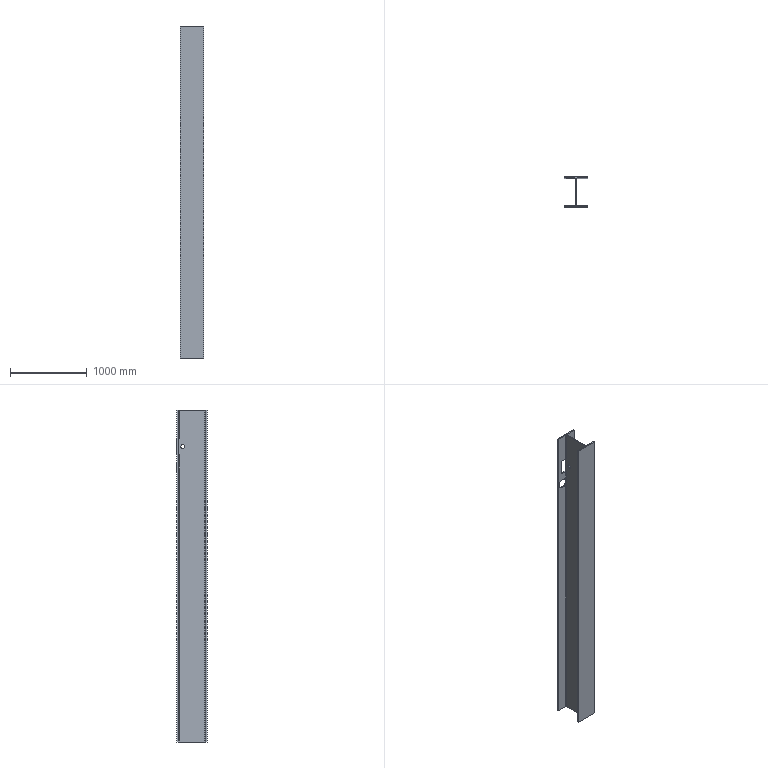Part | SolidWorks | features ICE 2, Extrusion 1 | 1 solid | 28 faces | box 300 x 390 x 4313 mm | volume 56956384 mm3 | plane 18 | cylinder 10 | commonest cylinder face diameters 26 x6 51 x2 125 x2
STEP:
#1=CARTESIAN_POINT('',(155.,289.5,3838.));
#2=VERTEX_POINT('',#1);
#3=CARTESIAN_POINT('',(155.,340.5,3838.));
#4=VERTEX_POINT('',#3);
#5=CARTESIAN_POINT('',(155.,315.,3838.));
#6=DIRECTION('',(1.,0.,0.));
#7=DIRECTION('',(0.,0.,1.));
#8=AXIS2_PLACEMENT_3D('',#5,#6,#7);
#9=CIRCLE('',#8,25.5);
#10=EDGE_CURVE('',#2,#4,#9,.T.);
#11=ORIENTED_EDGE('',*,*,#10,.T.);
#12=CARTESIAN_POINT('',(145.,340.5,3838.));
#13=VERTEX_POINT('',#12);
#14=CARTESIAN_POINT('',(300.001,340.5,3838.));
#15=DIRECTION('',(-1.,0.,0.));
#16=VECTOR('',#15,1000.);
#17=LINE('',#14,#16);
#18=EDGE_CURVE('',#4,#13,#17,.T.);
#19=ORIENTED_EDGE('',*,*,#18,.T.);
#20=CARTESIAN_POINT('',(145.,289.5,3838.));
#21=VERTEX_POINT('',#20);
#22=CARTESIAN_POINT('',(145.,315.,3838.));
#23=DIRECTION('',(-1.,0.,0.));
#24=DIRECTION('',(0.,-1.,0.));
#25=AXIS2_PLACEMENT_3D('',#22,#23,#24);
#26=CIRCLE('',#25,25.5);
#27=EDGE_CURVE('',#13,#21,#26,.T.);
#28=ORIENTED_EDGE('',*,*,#27,.T.);
#29=CARTESIAN_POINT('',(300.001,289.5,3838.));
#30=DIRECTION('',(-1.,0.,0.));
#31=VECTOR('',#30,1000.);
#32=LINE('',#29,#31);
#33=EDGE_CURVE('',#2,#21,#32,.T.);
#34=ORIENTED_EDGE('',*,*,#33,.F.);
#35=EDGE_LOOP('',(#11,#19,#28,#34));
#36=FACE_OUTER_BOUND('',#35,.T.);
#37=CARTESIAN_POINT('',(300.001,315.,3838.));
#38=DIRECTION('',(-1.,0.,0.));
#39=DIRECTION('',(0.,-1.,0.));
#40=AXIS2_PLACEMENT_3D('',#37,#38,#39);
#41=CYLINDRICAL_SURFACE('',#40,25.5);
#42=ADVANCED_FACE('',(#36),#41,.F.);
#43=CARTESIAN_POINT('',(85.,374.,3510.5));
#44=VERTEX_POINT('',#43);
#45=CARTESIAN_POINT('',(85.,374.,3635.5));
#46=VERTEX_POINT('',#45);
#47=CARTESIAN_POINT('',(85.,374.,3573.));
#48=DIRECTION('',(0.,1.,0.));
#49=DIRECTION('',(-1.,0.,0.));
#50=AXIS2_PLACEMENT_3D('',#47,#48,#49);
#51=CIRCLE('',#50,62.5);
#52=EDGE_CURVE('',#44,#46,#51,.T.);
#53=ORIENTED_EDGE('',*,*,#52,.F.);
#54=CARTESIAN_POINT('',(85.,390.,3510.5));
#55=VERTEX_POINT('',#54);
#56=CARTESIAN_POINT('',(85.,360.,3510.5));
#57=DIRECTION('',(0.,1.,0.));
#58=VECTOR('',#57,1000.);
#59=LINE('',#56,#58);
#60=EDGE_CURVE('',#44,#55,#59,.T.);
#61=ORIENTED_EDGE('',*,*,#60,.T.);
#62=CARTESIAN_POINT('',(85.,390.,3635.5));
#63=VERTEX_POINT('',#62);
#64=CARTESIAN_POINT('',(85.,390.,3573.));
#65=DIRECTION('',(0.,1.,0.));
#66=DIRECTION('',(0.,0.,1.));
#67=AXIS2_PLACEMENT_3D('',#64,#65,#66);
#68=CIRCLE('',#67,62.5);
#69=EDGE_CURVE('',#55,#63,#68,.T.);
#70=ORIENTED_EDGE('',*,*,#69,.T.);
#71=CARTESIAN_POINT('',(85.,360.,3635.5));
#72=DIRECTION('',(0.,1.,0.));
#73=VECTOR('',#72,1000.);
#74=LINE('',#71,#73);
#75=EDGE_CURVE('',#46,#63,#74,.T.);
#76=ORIENTED_EDGE('',*,*,#75,.F.);
#77=EDGE_LOOP('',(#53,#61,#70,#76));
#78=FACE_OUTER_BOUND('',#77,.T.);
#79=CARTESIAN_POINT('',(85.,360.,3573.));
#80=DIRECTION('',(0.,1.,0.));
#81=DIRECTION('',(0.,0.,1.));
#82=AXIS2_PLACEMENT_3D('',#79,#80,#81);
#83=CYLINDRICAL_SURFACE('',#82,62.5);
#84=ADVANCED_FACE('',(#78),#83,.F.);
#85=CARTESIAN_POINT('',(132.,374.,3738.));
#86=VERTEX_POINT('',#85);
#87=CARTESIAN_POINT('',(132.,374.,3614.198));
#88=VERTEX_POINT('',#87);
#89=CARTESIAN_POINT('',(132.,374.,4313.));
#90=DIRECTION('',(0.,0.,-1.));
#91=VECTOR('',#90,1000.);
#92=LINE('',#89,#91);
#93=EDGE_CURVE('',#86,#88,#92,.T.);
#94=ORIENTED_EDGE('',*,*,#93,.T.);
#95=CARTESIAN_POINT('',(145.,361.,3590.5));
#96=VERTEX_POINT('',#95);
#97=CARTESIAN_POINT('',(132.,374.,3614.198));
#98=CARTESIAN_POINT('',(132.872,374.,3613.203));
#99=CARTESIAN_POINT('',(133.708,373.913,3612.185));
#100=CARTESIAN_POINT('',(134.912,373.676,3610.623));
#101=CARTESIAN_POINT('',(135.304,373.579,3610.097));
#102=CARTESIAN_POINT('',(136.073,373.352,3609.032));
#103=CARTESIAN_POINT('',(136.447,373.222,3608.495));
#104=CARTESIAN_POINT('',(137.533,372.789,3606.885));
#105=CARTESIAN_POINT('',(138.212,372.445,3605.808));
#106=CARTESIAN_POINT('',(139.486,371.655,3603.644));
#107=CARTESIAN_POINT('',(140.082,371.21,3602.559));
#108=CARTESIAN_POINT('',(140.918,370.466,3600.925));
#109=CARTESIAN_POINT('',(141.187,370.206,3600.38));
#110=CARTESIAN_POINT('',(141.705,369.658,3599.29));
#111=CARTESIAN_POINT('',(141.955,369.369,3598.744));
#112=CARTESIAN_POINT('',(142.434,368.764,3597.657));
#113=CARTESIAN_POINT('',(142.662,368.448,3597.117));
#114=CARTESIAN_POINT('',(143.097,367.783,3596.049));
#115=CARTESIAN_POINT('',(143.305,367.433,3595.52));
#116=CARTESIAN_POINT('',(143.694,366.693,3594.483));
#117=CARTESIAN_POINT('',(143.877,366.304,3593.976));
#118=CARTESIAN_POINT('',(144.131,365.679,3593.245));
#119=CARTESIAN_POINT('',(144.212,365.463,3593.006));
#120=CARTESIAN_POINT('',(144.367,365.013,3592.54));
#121=CARTESIAN_POINT('',(144.441,364.778,3592.314));
#122=CARTESIAN_POINT('',(144.58,364.287,3591.881));
#123=CARTESIAN_POINT('',(144.645,364.032,3591.677));
#124=CARTESIAN_POINT('',(144.761,363.494,3591.299));
#125=CARTESIAN_POINT('',(144.814,363.21,3591.125));
#126=CARTESIAN_POINT('',(144.902,362.62,3590.833));
#127=CARTESIAN_POINT('',(144.938,362.313,3590.713));
#128=CARTESIAN_POINT('',(144.974,361.831,3590.588));
#129=CARTESIAN_POINT('',(144.984,361.665,3590.555));
#130=CARTESIAN_POINT('',(144.997,361.333,3590.511));
#131=CARTESIAN_POINT('',(145.,361.166,3590.5));
#132=CARTESIAN_POINT('',(145.,361.,3590.5));
#133=B_SPLINE_CURVE_WITH_KNOTS('',3,(#97,#98,#99,#100,#101,#102,#103,#104,#105,#106,#107,#108,#109,#110,#111,#112,#113,#114,#115,#116,#117,#118,#119,#120,#121,#122,#123,#124,#125,#126,#127,#128,#129,#130,#131,#132),.UNSPECIFIED.,.F.,.F.,(4,2,2,2,2,2,2,2,2,2,2,2,2,2,2,2,2,4),(0.02497,0.02896,0.03095,0.03294,0.03692,0.04091,0.0429,0.04489,0.04688,0.04888,0.05087,0.05187,0.05286,0.05386,0.05485,0.05585,0.05635,0.05685),.UNSPECIFIED.);
#134=EDGE_CURVE('',#88,#96,#133,.T.);
#135=ORIENTED_EDGE('',*,*,#134,.T.);
#136=CARTESIAN_POINT('',(145.,361.,3738.));
#137=VERTEX_POINT('',#136);
#138=CARTESIAN_POINT('',(145.,361.,4313.));
#139=DIRECTION('',(0.,0.,-1.));
#140=VECTOR('',#139,1000.);
#141=LINE('',#138,#140);
#142=EDGE_CURVE('',#137,#96,#141,.T.);
#143=ORIENTED_EDGE('',*,*,#142,.F.);
#144=CARTESIAN_POINT('',(132.,361.,3738.));
#145=DIRECTION('',(0.,0.,1.));
#146=DIRECTION('',(-1.,0.,0.));
#147=AXIS2_PLACEMENT_3D('',#144,#145,#146);
#148=CIRCLE('',#147,13.);
#149=EDGE_CURVE('',#137,#86,#148,.T.);
#150=ORIENTED_EDGE('',*,*,#149,.T.);
#151=EDGE_LOOP('',(#94,#135,#143,#150));
#152=FACE_OUTER_BOUND('',#151,.T.);
#153=CARTESIAN_POINT('',(132.,361.,4313.));
#154=DIRECTION('',(0.,0.,-1.));
#155=DIRECTION('',(-1.,0.,0.));
#156=AXIS2_PLACEMENT_3D('',#153,#154,#155);
#157=CYLINDRICAL_SURFACE('',#156,13.);
#158=ADVANCED_FACE('',(#152),#157,.F.);
#159=CARTESIAN_POINT('',(132.,374.,4313.));
#160=VERTEX_POINT('',#159);
#161=CARTESIAN_POINT('',(132.,374.,3938.));
#162=VERTEX_POINT('',#161);
#163=CARTESIAN_POINT('',(132.,374.,4313.));
#164=DIRECTION('',(0.,0.,-1.));
#165=VECTOR('',#164,1000.);
#166=LINE('',#163,#165);
#167=EDGE_CURVE('',#160,#162,#166,.T.);
#168=ORIENTED_EDGE('',*,*,#167,.T.);
#169=CARTESIAN_POINT('',(145.,361.,3938.));
#170=VERTEX_POINT('',#169);
#171=CARTESIAN_POINT('',(132.,361.,3938.));
#172=DIRECTION('',(0.,0.,-1.));
#173=DIRECTION('',(1.,0.,0.));
#174=AXIS2_PLACEMENT_3D('',#171,#172,#173);
#175=CIRCLE('',#174,13.);
#176=EDGE_CURVE('',#162,#170,#175,.T.);
#177=ORIENTED_EDGE('',*,*,#176,.T.);
#178=CARTESIAN_POINT('',(145.,361.,4313.));
#179=VERTEX_POINT('',#178);
#180=CARTESIAN_POINT('',(145.,361.,4313.));
#181=DIRECTION('',(0.,0.,-1.));
#182=VECTOR('',#181,1000.);
#183=LINE('',#180,#182);
#184=EDGE_CURVE('',#179,#170,#183,.T.);
#185=ORIENTED_EDGE('',*,*,#184,.F.);
#186=CARTESIAN_POINT('',(132.,361.,4313.));
#187=DIRECTION('',(0.,0.,-1.));
#188=DIRECTION('',(-1.,0.,0.));
#189=AXIS2_PLACEMENT_3D('',#186,#187,#188);
#190=CIRCLE('',#189,13.);
#191=EDGE_CURVE('',#160,#179,#190,.T.);
#192=ORIENTED_EDGE('',*,*,#191,.F.);
#193=EDGE_LOOP('',(#168,#177,#185,#192));
#194=FACE_OUTER_BOUND('',#193,.T.);
#195=CARTESIAN_POINT('',(132.,361.,4313.));
#196=DIRECTION('',(0.,0.,-1.));
#197=DIRECTION('',(-1.,0.,0.));
#198=AXIS2_PLACEMENT_3D('',#195,#196,#197);
#199=CYLINDRICAL_SURFACE('',#198,13.);
#200=ADVANCED_FACE('',(#194),#199,.F.);
#201=CARTESIAN_POINT('',(0.,16.,0.));
#202=VERTEX_POINT('',#201);
#203=CARTESIAN_POINT('',(0.,0.,0.));
#204=VERTEX_POINT('',#203);
#205=CARTESIAN_POINT('',(0.,16.,0.));
#206=DIRECTION('',(0.,-1.,0.));
#207=VECTOR('',#206,1000.);
#208=LINE('',#205,#207);
#209=EDGE_CURVE('',#202,#204,#208,.T.);
#210=ORIENTED_EDGE('',*,*,#209,.T.);
#211=CARTESIAN_POINT('',(0.,0.,4313.));
#212=VERTEX_POINT('',#211);
#213=CARTESIAN_POINT('',(0.,0.,4313.));
#214=DIRECTION('',(0.,0.,-1.));
#215=VECTOR('',#214,1000.);
#216=LINE('',#213,#215);
#217=EDGE_CURVE('',#212,#204,#216,.T.);
#218=ORIENTED_EDGE('',*,*,#217,.F.);
#219=CARTESIAN_POINT('',(0.,16.,4313.));
#220=VERTEX_POINT('',#219);
#221=CARTESIAN_POINT('',(0.,16.,4313.));
#222=DIRECTION('',(0.,-1.,0.));
#223=VECTOR('',#222,1000.);
#224=LINE('',#221,#223);
#225=EDGE_CURVE('',#220,#212,#224,.T.);
#226=ORIENTED_EDGE('',*,*,#225,.F.);
#227=CARTESIAN_POINT('',(0.,16.,4313.));
#228=DIRECTION('',(0.,0.,-1.));
#229=VECTOR('',#228,1000.);
#230=LINE('',#227,#229);
#231=EDGE_CURVE('',#220,#202,#230,.T.);
#232=ORIENTED_EDGE('',*,*,#231,.T.);
#233=EDGE_LOOP('',(#210,#218,#226,#232));
#234=FACE_OUTER_BOUND('',#233,.T.);
#235=CARTESIAN_POINT('',(0.,16.,4313.));
#236=DIRECTION('',(1.,0.,0.));
#237=DIRECTION('',(0.,1.,0.));
#238=AXIS2_PLACEMENT_3D('',#235,#236,#237);
#239=PLANE('',#238);
#240=ADVANCED_FACE('',(#234),#239,.F.);
#241=CARTESIAN_POINT('',(300.,0.,0.));
#242=VERTEX_POINT('',#241);
#243=CARTESIAN_POINT('',(0.,0.,0.));
#244=DIRECTION('',(1.,0.,0.));
#245=VECTOR('',#244,1000.);
#246=LINE('',#243,#245);
#247=EDGE_CURVE('',#204,#242,#246,.T.);
#248=ORIENTED_EDGE('',*,*,#247,.T.);
#249=CARTESIAN_POINT('',(300.,0.,4313.));
#250=VERTEX_POINT('',#249);
#251=CARTESIAN_POINT('',(300.,0.,4313.));
#252=DIRECTION('',(0.,0.,-1.));
#253=VECTOR('',#252,1000.);
#254=LINE('',#251,#253);
#255=EDGE_CURVE('',#250,#242,#254,.T.);
#256=ORIENTED_EDGE('',*,*,#255,.F.);
#257=CARTESIAN_POINT('',(0.,0.,4313.));
#258=DIRECTION('',(1.,0.,0.));
#259=VECTOR('',#258,1000.);
#260=LINE('',#257,#259);
#261=EDGE_CURVE('',#212,#250,#260,.T.);
#262=ORIENTED_EDGE('',*,*,#261,.F.);
#263=ORIENTED_EDGE('',*,*,#217,.T.);
#264=EDGE_LOOP('',(#248,#256,#262,#263));
#265=FACE_OUTER_BOUND('',#264,.T.);
#266=CARTESIAN_POINT('',(0.,0.,4313.));
#267=DIRECTION('',(0.,1.,0.));
#268=DIRECTION('',(0.,0.,1.));
#269=AXIS2_PLACEMENT_3D('',#266,#267,#268);
#270=PLANE('',#269);
#271=ADVANCED_FACE('',(#265),#270,.F.);
#272=CARTESIAN_POINT('',(300.,16.,0.));
#273=VERTEX_POINT('',#272);
#274=CARTESIAN_POINT('',(300.,0.,0.));
#275=DIRECTION('',(0.,1.,0.));
#276=VECTOR('',#275,1000.);
#277=LINE('',#274,#276);
#278=EDGE_CURVE('',#242,#273,#277,.T.);
#279=ORIENTED_EDGE('',*,*,#278,.T.);
#280=CARTESIAN_POINT('',(300.,16.,4313.));
#281=VERTEX_POINT('',#280);
#282=CARTESIAN_POINT('',(300.,16.,4313.));
#283=DIRECTION('',(0.,0.,-1.));
#284=VECTOR('',#283,1000.);
#285=LINE('',#282,#284);
#286=EDGE_CURVE('',#281,#273,#285,.T.);
#287=ORIENTED_EDGE('',*,*,#286,.F.);
#288=CARTESIAN_POINT('',(300.,0.,4313.));
#289=DIRECTION('',(0.,1.,0.));
#290=VECTOR('',#289,1000.);
#291=LINE('',#288,#290);
#292=EDGE_CURVE('',#250,#281,#291,.T.);
#293=ORIENTED_EDGE('',*,*,#292,.F.);
#294=ORIENTED_EDGE('',*,*,#255,.T.);
#295=EDGE_LOOP('',(#279,#287,#293,#294));
#296=FACE_OUTER_BOUND('',#295,.T.);
#297=CARTESIAN_POINT('',(300.,0.,4313.));
#298=DIRECTION('',(-1.,0.,0.));
#299=DIRECTION('',(0.,0.,1.));
#300=AXIS2_PLACEMENT_3D('',#297,#298,#299);
#301=PLANE('',#300);
#302=ADVANCED_FACE('',(#296),#301,.F.);
#303=CARTESIAN_POINT('',(168.,16.,0.));
#304=VERTEX_POINT('',#303);
#305=CARTESIAN_POINT('',(300.,16.,0.));
#306=DIRECTION('',(-1.,0.,0.));
#307=VECTOR('',#306,1000.);
#308=LINE('',#305,#307);
#309=EDGE_CURVE('',#273,#304,#308,.T.);
#310=ORIENTED_EDGE('',*,*,#309,.T.);
#311=CARTESIAN_POINT('',(168.,16.,4313.));
#312=VERTEX_POINT('',#311);
#313=CARTESIAN_POINT('',(168.,16.,4313.));
#314=DIRECTION('',(0.,0.,-1.));
#315=VECTOR('',#314,1000.);
#316=LINE('',#313,#315);
#317=EDGE_CURVE('',#312,#304,#316,.T.);
#318=ORIENTED_EDGE('',*,*,#317,.F.);
#319=CARTESIAN_POINT('',(300.,16.,4313.));
#320=DIRECTION('',(-1.,0.,0.));
#321=VECTOR('',#320,1000.);
#322=LINE('',#319,#321);
#323=EDGE_CURVE('',#281,#312,#322,.T.);
#324=ORIENTED_EDGE('',*,*,#323,.F.);
#325=ORIENTED_EDGE('',*,*,#286,.T.);
#326=EDGE_LOOP('',(#310,#318,#324,#325));
#327=FACE_OUTER_BOUND('',#326,.T.);
#328=CARTESIAN_POINT('',(300.,16.,4313.));
#329=DIRECTION('',(0.,-1.,0.));
#330=DIRECTION('',(1.,0.,0.));
#331=AXIS2_PLACEMENT_3D('',#328,#329,#330);
#332=PLANE('',#331);
#333=ADVANCED_FACE('',(#327),#332,.F.);
#334=CARTESIAN_POINT('',(155.,29.,0.));
#335=VERTEX_POINT('',#334);
#336=CARTESIAN_POINT('',(168.,29.,0.));
#337=DIRECTION('',(0.,0.,-1.));
#338=DIRECTION('',(-1.,0.,0.));
#339=AXIS2_PLACEMENT_3D('',#336,#337,#338);
#340=CIRCLE('',#339,13.);
#341=EDGE_CURVE('',#304,#335,#340,.T.);
#342=ORIENTED_EDGE('',*,*,#341,.T.);
#343=CARTESIAN_POINT('',(155.,29.,4313.));
#344=VERTEX_POINT('',#343);
#345=CARTESIAN_POINT('',(155.,29.,4313.));
#346=DIRECTION('',(0.,0.,-1.));
#347=VECTOR('',#346,1000.);
#348=LINE('',#345,#347);
#349=EDGE_CURVE('',#344,#335,#348,.T.);
#350=ORIENTED_EDGE('',*,*,#349,.F.);
#351=CARTESIAN_POINT('',(168.,29.,4313.));
#352=DIRECTION('',(0.,0.,-1.));
#353=DIRECTION('',(-1.,0.,0.));
#354=AXIS2_PLACEMENT_3D('',#351,#352,#353);
#355=CIRCLE('',#354,13.);
#356=EDGE_CURVE('',#312,#344,#355,.T.);
#357=ORIENTED_EDGE('',*,*,#356,.F.);
#358=ORIENTED_EDGE('',*,*,#317,.T.);
#359=EDGE_LOOP('',(#342,#350,#357,#358));
#360=FACE_OUTER_BOUND('',#359,.T.);
#361=CARTESIAN_POINT('',(168.,29.,4313.));
#362=DIRECTION('',(0.,0.,-1.));
#363=DIRECTION('',(-1.,0.,0.));
#364=AXIS2_PLACEMENT_3D('',#361,#362,#363);
#365=CYLINDRICAL_SURFACE('',#364,13.);
#366=ADVANCED_FACE('',(#360),#365,.F.);
#367=ORIENTED_EDGE('',*,*,#10,.F.);
#368=CARTESIAN_POINT('',(155.,315.,3838.));
#369=DIRECTION('',(1.,0.,0.));
#370=DIRECTION('',(0.,0.,1.));
#371=AXIS2_PLACEMENT_3D('',#368,#369,#370);
#372=CIRCLE('',#371,25.5);
#373=EDGE_CURVE('',#4,#2,#372,.T.);
#374=ORIENTED_EDGE('',*,*,#373,.F.);
#375=EDGE_LOOP('',(#367,#374));
#376=FACE_BOUND('',#375,.T.);
#377=CARTESIAN_POINT('',(155.,361.,0.));
#378=VERTEX_POINT('',#377);
#379=CARTESIAN_POINT('',(155.,29.,0.));
#380=DIRECTION('',(0.,1.,0.));
#381=VECTOR('',#380,1000.);
#382=LINE('',#379,#381);
#383=EDGE_CURVE('',#335,#378,#382,.T.);
#384=ORIENTED_EDGE('',*,*,#383,.T.);
#385=CARTESIAN_POINT('',(155.,361.,4313.));
#386=VERTEX_POINT('',#385);
#387=CARTESIAN_POINT('',(155.,361.,4313.));
#388=DIRECTION('',(0.,0.,-1.));
#389=VECTOR('',#388,1000.);
#390=LINE('',#387,#389);
#391=EDGE_CURVE('',#386,#378,#390,.T.);
#392=ORIENTED_EDGE('',*,*,#391,.F.);
#393=CARTESIAN_POINT('',(155.,29.,4313.));
#394=DIRECTION('',(0.,1.,0.));
#395=VECTOR('',#394,1000.);
#396=LINE('',#393,#395);
#397=EDGE_CURVE('',#344,#386,#396,.T.);
#398=ORIENTED_EDGE('',*,*,#397,.F.);
#399=ORIENTED_EDGE('',*,*,#349,.T.);
#400=EDGE_LOOP('',(#384,#392,#398,#399));
#401=FACE_OUTER_BOUND('',#400,.T.);
#402=CARTESIAN_POINT('',(155.,29.,4313.));
#403=DIRECTION('',(-1.,0.,0.));
#404=DIRECTION('',(0.,0.,1.));
#405=AXIS2_PLACEMENT_3D('',#402,#403,#404);
#406=PLANE('',#405);
#407=ADVANCED_FACE('',(#376,#401),#406,.F.);
#408=CARTESIAN_POINT('',(168.,374.,0.));
#409=VERTEX_POINT('',#408);
#410=CARTESIAN_POINT('',(168.,361.,0.));
#411=DIRECTION('',(0.,0.,-1.));
#412=DIRECTION('',(-1.,0.,0.));
#413=AXIS2_PLACEMENT_3D('',#410,#411,#412);
#414=CIRCLE('',#413,13.);
#415=EDGE_CURVE('',#378,#409,#414,.T.);
#416=ORIENTED_EDGE('',*,*,#415,.T.);
#417=CARTESIAN_POINT('',(168.,374.,4313.));
#418=VERTEX_POINT('',#417);
#419=CARTESIAN_POINT('',(168.,374.,4313.));
#420=DIRECTION('',(0.,0.,-1.));
#421=VECTOR('',#420,1000.);
#422=LINE('',#419,#421);
#423=EDGE_CURVE('',#418,#409,#422,.T.);
#424=ORIENTED_EDGE('',*,*,#423,.F.);
#425=CARTESIAN_POINT('',(168.,361.,4313.));
#426=DIRECTION('',(0.,0.,-1.));
#427=DIRECTION('',(-1.,0.,0.));
#428=AXIS2_PLACEMENT_3D('',#425,#426,#427);
#429=CIRCLE('',#428,13.);
#430=EDGE_CURVE('',#386,#418,#429,.T.);
#431=ORIENTED_EDGE('',*,*,#430,.F.);
#432=ORIENTED_EDGE('',*,*,#391,.T.);
#433=EDGE_LOOP('',(#416,#424,#431,#432));
#434=FACE_OUTER_BOUND('',#433,.T.);
#435=CARTESIAN_POINT('',(168.,361.,4313.));
#436=DIRECTION('',(0.,0.,-1.));
#437=DIRECTION('',(-1.,0.,0.));
#438=AXIS2_PLACEMENT_3D('',#435,#436,#437);
#439=CYLINDRICAL_SURFACE('',#438,13.);
#440=ADVANCED_FACE('',(#434),#439,.F.);
#441=CARTESIAN_POINT('',(300.,374.,0.));
#442=VERTEX_POINT('',#441);
#443=CARTESIAN_POINT('',(168.,374.,0.));
#444=DIRECTION('',(1.,0.,0.));
#445=VECTOR('',#444,1000.);
#446=LINE('',#443,#445);
#447=EDGE_CURVE('',#409,#442,#446,.T.);
#448=ORIENTED_EDGE('',*,*,#447,.T.);
#449=CARTESIAN_POINT('',(300.,374.,4313.));
#450=VERTEX_POINT('',#449);
#451=CARTESIAN_POINT('',(300.,374.,4313.));
#452=DIRECTION('',(0.,0.,-1.));
#453=VECTOR('',#452,1000.);
#454=LINE('',#451,#453);
#455=EDGE_CURVE('',#450,#442,#454,.T.);
#456=ORIENTED_EDGE('',*,*,#455,.F.);
#457=CARTESIAN_POINT('',(168.,374.,4313.));
#458=DIRECTION('',(1.,0.,0.));
#459=VECTOR('',#458,1000.);
#460=LINE('',#457,#459);
#461=EDGE_CURVE('',#418,#450,#460,.T.);
#462=ORIENTED_EDGE('',*,*,#461,.F.);
#463=ORIENTED_EDGE('',*,*,#423,.T.);
#464=EDGE_LOOP('',(#448,#456,#462,#463));
#465=FACE_OUTER_BOUND('',#464,.T.);
#466=CARTESIAN_POINT('',(168.,374.,4313.));
#467=DIRECTION('',(0.,1.,0.));
#468=DIRECTION('',(0.,0.,1.));
#469=AXIS2_PLACEMENT_3D('',#466,#467,#468);
#470=PLANE('',#469);
#471=ADVANCED_FACE('',(#465),#470,.F.);
#472=CARTESIAN_POINT('',(300.,390.,0.));
#473=VERTEX_POINT('',#472);
#474=CARTESIAN_POINT('',(300.,374.,0.));
#475=DIRECTION('',(0.,1.,0.));
#476=VECTOR('',#475,1000.);
#477=LINE('',#474,#476);
#478=EDGE_CURVE('',#442,#473,#477,.T.);
#479=ORIENTED_EDGE('',*,*,#478,.T.);
#480=CARTESIAN_POINT('',(300.,390.,4313.));
#481=VERTEX_POINT('',#480);
#482=CARTESIAN_POINT('',(300.,390.,4313.));
#483=DIRECTION('',(0.,0.,-1.));
#484=VECTOR('',#483,1000.);
#485=LINE('',#482,#484);
#486=EDGE_CURVE('',#481,#473,#485,.T.);
#487=ORIENTED_EDGE('',*,*,#486,.F.);
#488=CARTESIAN_POINT('',(300.,374.,4313.));
#489=DIRECTION('',(0.,1.,0.));
#490=VECTOR('',#489,1000.);
#491=LINE('',#488,#490);
#492=EDGE_CURVE('',#450,#481,#491,.T.);
#493=ORIENTED_EDGE('',*,*,#492,.F.);
#494=ORIENTED_EDGE('',*,*,#455,.T.);
#495=EDGE_LOOP('',(#479,#487,#493,#494));
#496=FACE_OUTER_BOUND('',#495,.T.);
#497=CARTESIAN_POINT('',(300.,374.,4313.));
#498=DIRECTION('',(-1.,0.,0.));
#499=DIRECTION('',(0.,-1.,0.));
#500=AXIS2_PLACEMENT_3D('',#497,#498,#499);
#501=PLANE('',#500);
#502=ADVANCED_FACE('',(#496),#501,.F.);
#503=CARTESIAN_POINT('',(85.,390.,3573.));
#504=DIRECTION('',(0.,1.,0.));
#505=DIRECTION('',(0.,0.,1.));
#506=AXIS2_PLACEMENT_3D('',#503,#504,#505);
#507=CIRCLE('',#506,62.5);
#508=EDGE_CURVE('',#63,#55,#507,.T.);
#509=ORIENTED_EDGE('',*,*,#508,.F.);
#510=ORIENTED_EDGE('',*,*,#69,.F.);
#511=EDGE_LOOP('',(#509,#510));
#512=FACE_BOUND('',#511,.T.);
#513=CARTESIAN_POINT('',(145.,390.,3738.));
#514=VERTEX_POINT('',#513);
#515=CARTESIAN_POINT('',(55.,390.,3738.));
#516=VERTEX_POINT('',#515);
#517=CARTESIAN_POINT('',(145.,390.,3738.));
#518=DIRECTION('',(-1.,0.,0.));
#519=VECTOR('',#518,1000.);
#520=LINE('',#517,#519);
#521=EDGE_CURVE('',#514,#516,#520,.T.);
#522=ORIENTED_EDGE('',*,*,#521,.F.);
#523=CARTESIAN_POINT('',(145.,390.,3938.));
#524=VERTEX_POINT('',#523);
#525=CARTESIAN_POINT('',(145.,390.,3738.));
#526=DIRECTION('',(0.,0.,-1.));
#527=VECTOR('',#526,1000.);
#528=LINE('',#525,#527);
#529=EDGE_CURVE('',#524,#514,#528,.T.);
#530=ORIENTED_EDGE('',*,*,#529,.F.);
#531=CARTESIAN_POINT('',(55.,390.,3938.));
#532=VERTEX_POINT('',#531);
#533=CARTESIAN_POINT('',(145.,390.,3938.));
#534=DIRECTION('',(1.,0.,0.));
#535=VECTOR('',#534,1000.);
#536=LINE('',#533,#535);
#537=EDGE_CURVE('',#532,#524,#536,.T.);
#538=ORIENTED_EDGE('',*,*,#537,.F.);
#539=CARTESIAN_POINT('',(55.,390.,3738.));
#540=DIRECTION('',(0.,0.,1.));
#541=VECTOR('',#540,1000.);
#542=LINE('',#539,#541);
#543=EDGE_CURVE('',#516,#532,#542,.T.);
#544=ORIENTED_EDGE('',*,*,#543,.F.);
#545=EDGE_LOOP('',(#522,#530,#538,#544));
#546=FACE_BOUND('',#545,.T.);
#547=CARTESIAN_POINT('',(0.,390.,0.));
#548=VERTEX_POINT('',#547);
#549=CARTESIAN_POINT('',(300.,390.,0.));
#550=DIRECTION('',(-1.,0.,0.));
#551=VECTOR('',#550,1000.);
#552=LINE('',#549,#551);
#553=EDGE_CURVE('',#473,#548,#552,.T.);
#554=ORIENTED_EDGE('',*,*,#553,.T.);
#555=CARTESIAN_POINT('',(0.,390.,4313.));
#556=VERTEX_POINT('',#555);
#557=CARTESIAN_POINT('',(0.,390.,4313.));
#558=DIRECTION('',(0.,0.,-1.));
#559=VECTOR('',#558,1000.);
#560=LINE('',#557,#559);
#561=EDGE_CURVE('',#556,#548,#560,.T.);
#562=ORIENTED_EDGE('',*,*,#561,.F.);
#563=CARTESIAN_POINT('',(300.,390.,4313.));
#564=DIRECTION('',(-1.,0.,0.));
#565=VECTOR('',#564,1000.);
#566=LINE('',#563,#565);
#567=EDGE_CURVE('',#481,#556,#566,.T.);
#568=ORIENTED_EDGE('',*,*,#567,.F.);
#569=ORIENTED_EDGE('',*,*,#486,.T.);
#570=EDGE_LOOP('',(#554,#562,#568,#569));
#571=FACE_OUTER_BOUND('',#570,.T.);
#572=CARTESIAN_POINT('',(300.,390.,4313.));
#573=DIRECTION('',(0.,-1.,0.));
#574=DIRECTION('',(0.,0.,-1.));
#575=AXIS2_PLACEMENT_3D('',#572,#573,#574);
#576=PLANE('',#575);
#577=ADVANCED_FACE('',(#512,#546,#571),#576,.F.);
#578=CARTESIAN_POINT('',(0.,374.,0.));
#579=VERTEX_POINT('',#578);
#580=CARTESIAN_POINT('',(0.,390.,0.));
#581=DIRECTION('',(0.,-1.,0.));
#582=VECTOR('',#581,1000.);
#583=LINE('',#580,#582);
#584=EDGE_CURVE('',#548,#579,#583,.T.);
#585=ORIENTED_EDGE('',*,*,#584,.T.);
#586=CARTESIAN_POINT('',(0.,374.,4313.));
#587=VERTEX_POINT('',#586);
#588=CARTESIAN_POINT('',(0.,374.,4313.));
#589=DIRECTION('',(0.,0.,-1.));
#590=VECTOR('',#589,1000.);
#591=LINE('',#588,#590);
#592=EDGE_CURVE('',#587,#579,#591,.T.);
#593=ORIENTED_EDGE('',*,*,#592,.F.);
#594=CARTESIAN_POINT('',(0.,390.,4313.));
#595=DIRECTION('',(0.,-1.,0.));
#596=VECTOR('',#595,1000.);
#597=LINE('',#594,#596);
#598=EDGE_CURVE('',#556,#587,#597,.T.);
#599=ORIENTED_EDGE('',*,*,#598,.F.);
#600=ORIENTED_EDGE('',*,*,#561,.T.);
#601=EDGE_LOOP('',(#585,#593,#599,#600));
#602=FACE_OUTER_BOUND('',#601,.T.);
#603=CARTESIAN_POINT('',(0.,390.,4313.));
#604=DIRECTION('',(1.,0.,0.));
#605=DIRECTION('',(0.,0.,-1.));
#606=AXIS2_PLACEMENT_3D('',#603,#604,#605);
#607=PLANE('',#606);
#608=ADVANCED_FACE('',(#602),#607,.F.);
#609=CARTESIAN_POINT('',(132.,374.,3531.802));
#610=VERTEX_POINT('',#609);
#611=CARTESIAN_POINT('',(132.,374.,0.));
#612=VERTEX_POINT('',#611);
#613=CARTESIAN_POINT('',(132.,374.,4313.));
#614=DIRECTION('',(0.,0.,-1.));
#615=VECTOR('',#614,1000.);
#616=LINE('',#613,#615);
#617=EDGE_CURVE('',#610,#612,#616,.T.);
#618=ORIENTED_EDGE('',*,*,#617,.F.);
#619=CARTESIAN_POINT('',(85.,374.,3573.));
#620=DIRECTION('',(0.,1.,0.));
#621=DIRECTION('',(-1.,0.,0.));
#622=AXIS2_PLACEMENT_3D('',#619,#620,#621);
#623=CIRCLE('',#622,62.5);
#624=EDGE_CURVE('',#610,#44,#623,.T.);
#625=ORIENTED_EDGE('',*,*,#624,.T.);
#626=ORIENTED_EDGE('',*,*,#52,.T.);
#627=CARTESIAN_POINT('',(85.,374.,3573.));
#628=DIRECTION('',(0.,1.,0.));
#629=DIRECTION('',(-1.,0.,0.));
#630=AXIS2_PLACEMENT_3D('',#627,#628,#629);
#631=CIRCLE('',#630,62.5);
#632=EDGE_CURVE('',#46,#88,#631,.T.);
#633=ORIENTED_EDGE('',*,*,#632,.T.);
#634=ORIENTED_EDGE('',*,*,#93,.F.);
#635=CARTESIAN_POINT('',(55.,374.,3738.));
#636=VERTEX_POINT('',#635);
#637=CARTESIAN_POINT('',(0.,374.,3738.));
#638=DIRECTION('',(-1.,0.,0.));
#639=VECTOR('',#638,1000.);
#640=LINE('',#637,#639);
#641=EDGE_CURVE('',#86,#636,#640,.T.);
#642=ORIENTED_EDGE('',*,*,#641,.T.);
#643=CARTESIAN_POINT('',(55.,374.,3938.));
#644=VERTEX_POINT('',#643);
#645=CARTESIAN_POINT('',(55.,374.,4313.));
#646=DIRECTION('',(0.,0.,1.));
#647=VECTOR('',#646,1000.);
#648=LINE('',#645,#647);
#649=EDGE_CURVE('',#636,#644,#648,.T.);
#650=ORIENTED_EDGE('',*,*,#649,.T.);
#651=CARTESIAN_POINT('',(0.,374.,3938.));
#652=DIRECTION('',(1.,0.,0.));
#653=VECTOR('',#652,1000.);
#654=LINE('',#651,#653);
#655=EDGE_CURVE('',#644,#162,#654,.T.);
#656=ORIENTED_EDGE('',*,*,#655,.T.);
#657=ORIENTED_EDGE('',*,*,#167,.F.);
#658=CARTESIAN_POINT('',(0.,374.,4313.));
#659=DIRECTION('',(1.,0.,0.));
#660=VECTOR('',#659,1000.);
#661=LINE('',#658,#660);
#662=EDGE_CURVE('',#587,#160,#661,.T.);
#663=ORIENTED_EDGE('',*,*,#662,.F.);
#664=ORIENTED_EDGE('',*,*,#592,.T.);
#665=CARTESIAN_POINT('',(0.,374.,0.));
#666=DIRECTION('',(1.,0.,0.));
#667=VECTOR('',#666,1000.);
#668=LINE('',#665,#667);
#669=EDGE_CURVE('',#579,#612,#668,.T.);
#670=ORIENTED_EDGE('',*,*,#669,.T.);
#671=EDGE_LOOP('',(#618,#625,#626,#633,#634,#642,#650,#656,#657,#663,#664,#670));
#672=FACE_OUTER_BOUND('',#671,.T.);
#673=CARTESIAN_POINT('',(0.,374.,4313.));
#674=DIRECTION('',(0.,1.,0.));
#675=DIRECTION('',(-1.,0.,0.));
#676=AXIS2_PLACEMENT_3D('',#673,#674,#675);
#677=PLANE('',#676);
#678=ADVANCED_FACE('',(#672),#677,.F.);
#679=CARTESIAN_POINT('',(145.,361.,3555.5));
#680=VERTEX_POINT('',#679);
#681=CARTESIAN_POINT('',(145.,361.,0.));
#682=VERTEX_POINT('',#681);
#683=CARTESIAN_POINT('',(145.,361.,4313.));
#684=DIRECTION('',(0.,0.,-1.));
#685=VECTOR('',#684,1000.);
#686=LINE('',#683,#685);
#687=EDGE_CURVE('',#680,#682,#686,.T.);
#688=ORIENTED_EDGE('',*,*,#687,.F.);
#689=CARTESIAN_POINT('',(145.,361.,3555.5));
#690=CARTESIAN_POINT('',(145.,361.168,3555.5));
#691=CARTESIAN_POINT('',(144.997,361.338,3555.489));
#692=CARTESIAN_POINT('',(144.984,361.672,3555.444));
#693=CARTESIAN_POINT('',(144.974,361.837,3555.411));
#694=CARTESIAN_POINT('',(144.937,362.322,3555.284));
#695=CARTESIAN_POINT('',(144.9,362.638,3555.16));
#696=CARTESIAN_POINT('',(144.81,363.232,3554.862));
#697=CARTESIAN_POINT('',(144.758,363.513,3554.689));
#698=CARTESIAN_POINT('',(144.64,364.051,3554.308));
#699=CARTESIAN_POINT('',(144.574,364.31,3554.1));
#700=CARTESIAN_POINT('',(144.365,365.046,3553.449));
#701=CARTESIAN_POINT('',(144.209,365.488,3552.979));
#702=CARTESIAN_POINT('',(143.87,366.321,3552.003));
#703=CARTESIAN_POINT('',(143.687,366.709,3551.496));
#704=CARTESIAN_POINT('',(143.296,367.448,3550.458));
#705=CARTESIAN_POINT('',(143.088,367.798,3549.927));
#706=CARTESIAN_POINT('',(142.653,368.462,3548.86));
#707=CARTESIAN_POINT('',(142.425,368.776,3548.323));
#708=CARTESIAN_POINT('',(141.712,369.676,3546.705));
#709=CARTESIAN_POINT('',(141.196,370.22,3545.617));
#710=CARTESIAN_POINT('',(140.079,371.212,3543.435));
#711=CARTESIAN_POINT('',(139.478,371.661,3542.34));
#712=CARTESIAN_POINT('',(138.185,372.46,3540.149));
#713=CARTESIAN_POINT('',(137.503,372.803,3539.069));
#714=CARTESIAN_POINT('',(136.064,373.373,3536.94));
#715=CARTESIAN_POINT('',(135.308,373.598,3535.891));
#716=CARTESIAN_POINT('',(133.715,373.912,3533.824));
#717=CARTESIAN_POINT('',(132.879,374.,3532.806));
#718=CARTESIAN_POINT('',(132.,374.,3531.802));
#719=B_SPLINE_CURVE_WITH_KNOTS('',3,(#689,#690,#691,#692,#693,#694,#695,#696,#697,#698,#699,#700,#701,#702,#703,#704,#705,#706,#707,#708,#709,#710,#711,#712,#713,#714,#715,#716,#717,#718),.UNSPECIFIED.,.F.,.F.,(4,2,2,2,2,2,2,2,2,2,2,2,2,2,4),(0.001009,0.00151,0.002012,0.003016,0.00402,0.005023,0.007031,0.009038,0.01105,0.01305,0.01707,0.02108,0.0251,0.02911,0.03313),.UNSPECIFIED.);
#720=EDGE_CURVE('',#680,#610,#719,.T.);
#721=ORIENTED_EDGE('',*,*,#720,.T.);
#722=ORIENTED_EDGE('',*,*,#617,.T.);
#723=CARTESIAN_POINT('',(132.,361.,0.));
#724=DIRECTION('',(0.,0.,-1.));
#725=DIRECTION('',(-1.,0.,0.));
#726=AXIS2_PLACEMENT_3D('',#723,#724,#725);
#727=CIRCLE('',#726,13.);
#728=EDGE_CURVE('',#612,#682,#727,.T.);
#729=ORIENTED_EDGE('',*,*,#728,.T.);
#730=EDGE_LOOP('',(#688,#721,#722,#729));
#731=FACE_OUTER_BOUND('',#730,.T.);
#732=CARTESIAN_POINT('',(132.,361.,4313.));
#733=DIRECTION('',(0.,0.,-1.));
#734=DIRECTION('',(-1.,0.,0.));
#735=AXIS2_PLACEMENT_3D('',#732,#733,#734);
#736=CYLINDRICAL_SURFACE('',#735,13.);
#737=ADVANCED_FACE('',(#731),#736,.F.);
#738=CARTESIAN_POINT('',(145.,315.,3838.));
#739=DIRECTION('',(-1.,0.,0.));
#740=DIRECTION('',(0.,-1.,0.));
#741=AXIS2_PLACEMENT_3D('',#738,#739,#740);
#742=CIRCLE('',#741,25.5);
#743=EDGE_CURVE('',#21,#13,#742,.T.);
#744=ORIENTED_EDGE('',*,*,#743,.F.);
#745=ORIENTED_EDGE('',*,*,#27,.F.);
#746=EDGE_LOOP('',(#744,#745));
#747=FACE_BOUND('',#746,.T.);
#748=ORIENTED_EDGE('',*,*,#184,.T.);
#749=CARTESIAN_POINT('',(145.,360.,3938.));
#750=DIRECTION('',(0.,1.,0.));
#751=VECTOR('',#750,1000.);
#752=LINE('',#749,#751);
#753=EDGE_CURVE('',#170,#524,#752,.T.);
#754=ORIENTED_EDGE('',*,*,#753,.T.);
#755=ORIENTED_EDGE('',*,*,#529,.T.);
#756=CARTESIAN_POINT('',(145.,360.,3738.));
#757=DIRECTION('',(0.,1.,0.));
#758=VECTOR('',#757,1000.);
#759=LINE('',#756,#758);
#760=EDGE_CURVE('',#137,#514,#759,.T.);
#761=ORIENTED_EDGE('',*,*,#760,.F.);
#762=ORIENTED_EDGE('',*,*,#142,.T.);
#763=CARTESIAN_POINT('',(145.,360.,3590.5));
#764=VERTEX_POINT('',#763);
#765=CARTESIAN_POINT('',(145.,360.,3590.5));
#766=DIRECTION('',(0.,-1.,0.));
#767=VECTOR('',#766,1000.);
#768=LINE('',#765,#767);
#769=EDGE_CURVE('',#96,#764,#768,.T.);
#770=ORIENTED_EDGE('',*,*,#769,.T.);
#771=CARTESIAN_POINT('',(145.,360.,3555.5));
#772=VERTEX_POINT('',#771);
#773=CARTESIAN_POINT('',(145.,360.,4313.));
#774=DIRECTION('',(0.,0.,1.));
#775=VECTOR('',#774,1000.);
#776=LINE('',#773,#775);
#777=EDGE_CURVE('',#772,#764,#776,.T.);
#778=ORIENTED_EDGE('',*,*,#777,.F.);
#779=CARTESIAN_POINT('',(145.,360.,3555.5));
#780=DIRECTION('',(0.,1.,0.));
#781=VECTOR('',#780,1000.);
#782=LINE('',#779,#781);
#783=EDGE_CURVE('',#772,#680,#782,.T.);
#784=ORIENTED_EDGE('',*,*,#783,.T.);
#785=ORIENTED_EDGE('',*,*,#687,.T.);
#786=CARTESIAN_POINT('',(145.,29.,0.));
#787=VERTEX_POINT('',#786);
#788=CARTESIAN_POINT('',(145.,361.,0.));
#789=DIRECTION('',(0.,-1.,0.));
#790=VECTOR('',#789,1000.);
#791=LINE('',#788,#790);
#792=EDGE_CURVE('',#682,#787,#791,.T.);
#793=ORIENTED_EDGE('',*,*,#792,.T.);
#794=CARTESIAN_POINT('',(145.,29.,4313.));
#795=VERTEX_POINT('',#794);
#796=CARTESIAN_POINT('',(145.,29.,4313.));
#797=DIRECTION('',(0.,0.,-1.));
#798=VECTOR('',#797,1000.);
#799=LINE('',#796,#798);
#800=EDGE_CURVE('',#795,#787,#799,.T.);
#801=ORIENTED_EDGE('',*,*,#800,.F.);
#802=CARTESIAN_POINT('',(145.,361.,4313.));
#803=DIRECTION('',(0.,-1.,0.));
#804=VECTOR('',#803,1000.);
#805=LINE('',#802,#804);
#806=EDGE_CURVE('',#179,#795,#805,.T.);
#807=ORIENTED_EDGE('',*,*,#806,.F.);
#808=EDGE_LOOP('',(#748,#754,#755,#761,#762,#770,#778,#784,#785,#793,#801,#807));
#809=FACE_OUTER_BOUND('',#808,.T.);
#810=CARTESIAN_POINT('',(145.,361.,4313.));
#811=DIRECTION('',(1.,0.,0.));
#812=DIRECTION('',(0.,1.,0.));
#813=AXIS2_PLACEMENT_3D('',#810,#811,#812);
#814=PLANE('',#813);
#815=ADVANCED_FACE('',(#747,#809),#814,.F.);
#816=CARTESIAN_POINT('',(132.,16.,0.));
#817=VERTEX_POINT('',#816);
#818=CARTESIAN_POINT('',(132.,29.,0.));
#819=DIRECTION('',(0.,0.,-1.));
#820=DIRECTION('',(-1.,0.,0.));
#821=AXIS2_PLACEMENT_3D('',#818,#819,#820);
#822=CIRCLE('',#821,13.);
#823=EDGE_CURVE('',#787,#817,#822,.T.);
#824=ORIENTED_EDGE('',*,*,#823,.T.);
#825=CARTESIAN_POINT('',(132.,16.,4313.));
#826=VERTEX_POINT('',#825);
#827=CARTESIAN_POINT('',(132.,16.,4313.));
#828=DIRECTION('',(0.,0.,-1.));
#829=VECTOR('',#828,1000.);
#830=LINE('',#827,#829);
#831=EDGE_CURVE('',#826,#817,#830,.T.);
#832=ORIENTED_EDGE('',*,*,#831,.F.);
#833=CARTESIAN_POINT('',(132.,29.,4313.));
#834=DIRECTION('',(0.,0.,-1.));
#835=DIRECTION('',(-1.,0.,0.));
#836=AXIS2_PLACEMENT_3D('',#833,#834,#835);
#837=CIRCLE('',#836,13.);
#838=EDGE_CURVE('',#795,#826,#837,.T.);
#839=ORIENTED_EDGE('',*,*,#838,.F.);
#840=ORIENTED_EDGE('',*,*,#800,.T.);
#841=EDGE_LOOP('',(#824,#832,#839,#840));
#842=FACE_OUTER_BOUND('',#841,.T.);
#843=CARTESIAN_POINT('',(132.,29.,4313.));
#844=DIRECTION('',(0.,0.,-1.));
#845=DIRECTION('',(-1.,0.,0.));
#846=AXIS2_PLACEMENT_3D('',#843,#844,#845);
#847=CYLINDRICAL_SURFACE('',#846,13.);
#848=ADVANCED_FACE('',(#842),#847,.F.);
#849=CARTESIAN_POINT('',(132.,16.,0.));
#850=DIRECTION('',(-1.,0.,0.));
#851=VECTOR('',#850,1000.);
#852=LINE('',#849,#851);
#853=EDGE_CURVE('',#817,#202,#852,.T.);
#854=ORIENTED_EDGE('',*,*,#853,.T.);
#855=ORIENTED_EDGE('',*,*,#231,.F.);
#856=CARTESIAN_POINT('',(132.,16.,4313.));
#857=DIRECTION('',(-1.,0.,0.));
#858=VECTOR('',#857,1000.);
#859=LINE('',#856,#858);
#860=EDGE_CURVE('',#826,#220,#859,.T.);
#861=ORIENTED_EDGE('',*,*,#860,.F.);
#862=ORIENTED_EDGE('',*,*,#831,.T.);
#863=EDGE_LOOP('',(#854,#855,#861,#862));
#864=FACE_OUTER_BOUND('',#863,.T.);
#865=CARTESIAN_POINT('',(132.,16.,4313.));
#866=DIRECTION('',(0.,-1.,0.));
#867=DIRECTION('',(1.,0.,0.));
#868=AXIS2_PLACEMENT_3D('',#865,#866,#867);
#869=PLANE('',#868);
#870=ADVANCED_FACE('',(#864),#869,.F.);
#871=ORIENTED_EDGE('',*,*,#225,.T.);
#872=ORIENTED_EDGE('',*,*,#261,.T.);
#873=ORIENTED_EDGE('',*,*,#292,.T.);
#874=ORIENTED_EDGE('',*,*,#323,.T.);
#875=ORIENTED_EDGE('',*,*,#356,.T.);
#876=ORIENTED_EDGE('',*,*,#397,.T.);
#877=ORIENTED_EDGE('',*,*,#430,.T.);
#878=ORIENTED_EDGE('',*,*,#461,.T.);
#879=ORIENTED_EDGE('',*,*,#492,.T.);
#880=ORIENTED_EDGE('',*,*,#567,.T.);
#881=ORIENTED_EDGE('',*,*,#598,.T.);
#882=ORIENTED_EDGE('',*,*,#662,.T.);
#883=ORIENTED_EDGE('',*,*,#191,.T.);
#884=ORIENTED_EDGE('',*,*,#806,.T.);
#885=ORIENTED_EDGE('',*,*,#838,.T.);
#886=ORIENTED_EDGE('',*,*,#860,.T.);
#887=EDGE_LOOP('',(#871,#872,#873,#874,#875,#876,#877,#878,#879,#880,#881,#882,#883,#884,#885,#886));
#888=FACE_OUTER_BOUND('',#887,.T.);
#889=CARTESIAN_POINT('',(168.,29.,4313.));
#890=DIRECTION('',(0.,0.,-1.));
#891=DIRECTION('',(-1.,0.,0.));
#892=AXIS2_PLACEMENT_3D('',#889,#890,#891);
#893=PLANE('',#892);
#894=ADVANCED_FACE('',(#888),#893,.F.);
#895=ORIENTED_EDGE('',*,*,#209,.F.);
#896=ORIENTED_EDGE('',*,*,#853,.F.);
#897=ORIENTED_EDGE('',*,*,#823,.F.);
#898=ORIENTED_EDGE('',*,*,#792,.F.);
#899=ORIENTED_EDGE('',*,*,#728,.F.);
#900=ORIENTED_EDGE('',*,*,#669,.F.);
#901=ORIENTED_EDGE('',*,*,#584,.F.);
#902=ORIENTED_EDGE('',*,*,#553,.F.);
#903=ORIENTED_EDGE('',*,*,#478,.F.);
#904=ORIENTED_EDGE('',*,*,#447,.F.);
#905=ORIENTED_EDGE('',*,*,#415,.F.);
#906=ORIENTED_EDGE('',*,*,#383,.F.);
#907=ORIENTED_EDGE('',*,*,#341,.F.);
#908=ORIENTED_EDGE('',*,*,#309,.F.);
#909=ORIENTED_EDGE('',*,*,#278,.F.);
#910=ORIENTED_EDGE('',*,*,#247,.F.);
#911=EDGE_LOOP('',(#895,#896,#897,#898,#899,#900,#901,#902,#903,#904,#905,#906,#907,#908,#909,#910));
#912=FACE_OUTER_BOUND('',#911,.T.);
#913=CARTESIAN_POINT('',(168.,29.,0.));
#914=DIRECTION('',(0.,0.,-1.));
#915=DIRECTION('',(-1.,0.,0.));
#916=AXIS2_PLACEMENT_3D('',#913,#914,#915);
#917=PLANE('',#916);
#918=ADVANCED_FACE('',(#912),#917,.T.);
#919=ORIENTED_EDGE('',*,*,#60,.F.);
#920=ORIENTED_EDGE('',*,*,#624,.F.);
#921=ORIENTED_EDGE('',*,*,#720,.F.);
#922=ORIENTED_EDGE('',*,*,#783,.F.);
#923=CARTESIAN_POINT('',(85.,360.,3573.));
#924=DIRECTION('',(0.,1.,0.));
#925=DIRECTION('',(0.,0.,1.));
#926=AXIS2_PLACEMENT_3D('',#923,#924,#925);
#927=CIRCLE('',#926,62.5);
#928=EDGE_CURVE('',#764,#772,#927,.T.);
#929=ORIENTED_EDGE('',*,*,#928,.F.);
#930=ORIENTED_EDGE('',*,*,#769,.F.);
#931=ORIENTED_EDGE('',*,*,#134,.F.);
#932=ORIENTED_EDGE('',*,*,#632,.F.);
#933=ORIENTED_EDGE('',*,*,#75,.T.);
#934=ORIENTED_EDGE('',*,*,#508,.T.);
#935=EDGE_LOOP('',(#919,#920,#921,#922,#929,#930,#931,#932,#933,#934));
#936=FACE_OUTER_BOUND('',#935,.T.);
#937=CARTESIAN_POINT('',(85.,360.,3573.));
#938=DIRECTION('',(0.,1.,0.));
#939=DIRECTION('',(0.,0.,1.));
#940=AXIS2_PLACEMENT_3D('',#937,#938,#939);
#941=CYLINDRICAL_SURFACE('',#940,62.5);
#942=ADVANCED_FACE('',(#936),#941,.F.);
#943=ORIENTED_EDGE('',*,*,#777,.T.);
#944=ORIENTED_EDGE('',*,*,#928,.T.);
#945=EDGE_LOOP('',(#943,#944));
#946=FACE_OUTER_BOUND('',#945,.T.);
#947=CARTESIAN_POINT('',(85.,360.,3573.));
#948=DIRECTION('',(0.,1.,0.));
#949=DIRECTION('',(0.,0.,1.));
#950=AXIS2_PLACEMENT_3D('',#947,#948,#949);
#951=PLANE('',#950);
#952=ADVANCED_FACE('',(#946),#951,.T.);
#953=CARTESIAN_POINT('',(55.,360.,3738.));
#954=DIRECTION('',(0.,1.,0.));
#955=VECTOR('',#954,1000.);
#956=LINE('',#953,#955);
#957=EDGE_CURVE('',#636,#516,#956,.T.);
#958=ORIENTED_EDGE('',*,*,#957,.T.);
#959=ORIENTED_EDGE('',*,*,#543,.T.);
#960=CARTESIAN_POINT('',(55.,360.,3938.));
#961=DIRECTION('',(0.,1.,0.));
#962=VECTOR('',#961,1000.);
#963=LINE('',#960,#962);
#964=EDGE_CURVE('',#644,#532,#963,.T.);
#965=ORIENTED_EDGE('',*,*,#964,.F.);
#966=ORIENTED_EDGE('',*,*,#649,.F.);
#967=EDGE_LOOP('',(#958,#959,#965,#966));
#968=FACE_OUTER_BOUND('',#967,.T.);
#969=CARTESIAN_POINT('',(55.,360.,3738.));
#970=DIRECTION('',(-1.,0.,0.));
#971=DIRECTION('',(0.,0.,1.));
#972=AXIS2_PLACEMENT_3D('',#969,#970,#971);
#973=PLANE('',#972);
#974=ADVANCED_FACE('',(#968),#973,.F.);
#975=ORIENTED_EDGE('',*,*,#964,.T.);
#976=ORIENTED_EDGE('',*,*,#537,.T.);
#977=ORIENTED_EDGE('',*,*,#753,.F.);
#978=ORIENTED_EDGE('',*,*,#176,.F.);
#979=ORIENTED_EDGE('',*,*,#655,.F.);
#980=EDGE_LOOP('',(#975,#976,#977,#978,#979));
#981=FACE_OUTER_BOUND('',#980,.T.);
#982=CARTESIAN_POINT('',(145.,360.,3938.));
#983=DIRECTION('',(0.,0.,1.));
#984=DIRECTION('',(1.,0.,0.));
#985=AXIS2_PLACEMENT_3D('',#982,#983,#984);
#986=PLANE('',#985);
#987=ADVANCED_FACE('',(#981),#986,.F.);
#988=ORIENTED_EDGE('',*,*,#149,.F.);
#989=ORIENTED_EDGE('',*,*,#760,.T.);
#990=ORIENTED_EDGE('',*,*,#521,.T.);
#991=ORIENTED_EDGE('',*,*,#957,.F.);
#992=ORIENTED_EDGE('',*,*,#641,.F.);
#993=EDGE_LOOP('',(#988,#989,#990,#991,#992));
#994=FACE_OUTER_BOUND('',#993,.T.);
#995=CARTESIAN_POINT('',(145.,360.,3738.));
#996=DIRECTION('',(0.,0.,-1.));
#997=DIRECTION('',(-1.,0.,0.));
#998=AXIS2_PLACEMENT_3D('',#995,#996,#997);
#999=PLANE('',#998);
#1000=ADVANCED_FACE('',(#994),#999,.F.);
#1001=ORIENTED_EDGE('',*,*,#18,.F.);
#1002=ORIENTED_EDGE('',*,*,#373,.T.);
#1003=ORIENTED_EDGE('',*,*,#33,.T.);
#1004=ORIENTED_EDGE('',*,*,#743,.T.);
#1005=EDGE_LOOP('',(#1001,#1002,#1003,#1004));
#1006=FACE_OUTER_BOUND('',#1005,.T.);
#1007=CARTESIAN_POINT('',(300.001,315.,3838.));
#1008=DIRECTION('',(-1.,0.,0.));
#1009=DIRECTION('',(0.,-1.,0.));
#1010=AXIS2_PLACEMENT_3D('',#1007,#1008,#1009);
#1011=CYLINDRICAL_SURFACE('',#1010,25.5);
#1012=ADVANCED_FACE('',(#1006),#1011,.F.);
#1013=CLOSED_SHELL('',(#42,#84,#158,#200,#240,#271,#302,#333,#366,#407,#440,#471,#502,#577,#608,#678,#737,#815,#848,#870,#894,#918,#942,#952,#974,#987,#1000,#1012));
#1014=MANIFOLD_SOLID_BREP('',#1013);
#1015=CARTESIAN_POINT('',(0.,0.,0.));
#1016=DIRECTION('',(0.,0.,1.));
#1017=DIRECTION('',(1.,0.,0.));
#1018=AXIS2_PLACEMENT_3D('',#1015,#1016,#1017);
#1019=(LENGTH_UNIT()NAMED_UNIT(*)SI_UNIT(.MILLI.,.METRE.));
#1020=UNCERTAINTY_MEASURE_WITH_UNIT(LENGTH_MEASURE(0.00001),#1019,'','');
#1021=(NAMED_UNIT(*)PLANE_ANGLE_UNIT()SI_UNIT($,.RADIAN.));
#1022=(NAMED_UNIT(*)SI_UNIT($,.STERADIAN.)SOLID_ANGLE_UNIT());
#1023=(GEOMETRIC_REPRESENTATION_CONTEXT(3)GLOBAL_UNCERTAINTY_ASSIGNED_CONTEXT((#1020))GLOBAL_UNIT_ASSIGNED_CONTEXT((#1019,#1021,#1022))REPRESENTATION_CONTEXT('',''));
#1024=ADVANCED_BREP_SHAPE_REPRESENTATION('',(#1014,#1018),#1023);